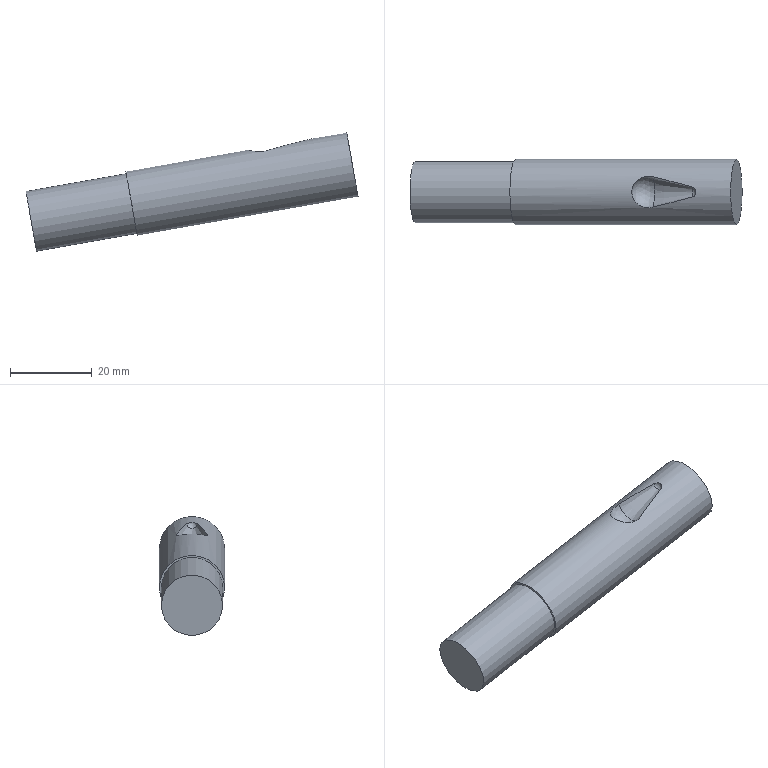Part | NX | features solid 2 | 1 solid | 8 faces | box 81.476 x 16 x 29.156 mm | volume 15288 mm3 | plane 3 | cylinder 2 | sphere 2 | cone 1 | commonest cylinder face diameters 15 x1 16 x1
STEP:
#1=CARTESIAN_POINT('',(-459.592,-11.393,50.494));
#2=VERTEX_POINT('',#1);
#3=CARTESIAN_POINT('',(-449.889,-8.922,53.051));
#4=VERTEX_POINT('',#3);
#5=CARTESIAN_POINT('',(-459.592,-11.393,50.494));
#6=CARTESIAN_POINT('',(-456.385,-10.61,51.483));
#7=CARTESIAN_POINT('',(-453.15,-9.775,52.335));
#8=CARTESIAN_POINT('',(-449.889,-8.922,53.051));
#9=B_SPLINE_CURVE_WITH_KNOTS('',3,(#5,#6,#7,#8),.UNSPECIFIED.,.F.,.F.,(4,4),(0.000000207,0.01034),.UNSPECIFIED.);
#10=EDGE_CURVE('',#2,#4,#9,.T.);
#11=ORIENTED_EDGE('',*,*,#10,.F.);
#12=CARTESIAN_POINT('',(-459.592,-3.877,50.494));
#13=VERTEX_POINT('',#12);
#14=CARTESIAN_POINT('',(-459.592,-3.877,50.494));
#15=CARTESIAN_POINT('',(-460.738,-3.598,50.141));
#16=CARTESIAN_POINT('',(-462.709,-3.96,50.065));
#17=CARTESIAN_POINT('',(-464.373,-5.808,50.453));
#18=CARTESIAN_POINT('',(-464.832,-7.629,50.597));
#19=CARTESIAN_POINT('',(-464.374,-9.46,50.454));
#20=CARTESIAN_POINT('',(-462.714,-11.307,50.066));
#21=CARTESIAN_POINT('',(-460.739,-11.672,50.141));
#22=CARTESIAN_POINT('',(-459.592,-11.393,50.494));
#23=B_SPLINE_CURVE_WITH_KNOTS('',3,(#14,#15,#16,#17,#18,#19,#20,#21,#22),.UNSPECIFIED.,.F.,.F.,(4,1,1,1,1,1,4),(0.000000204,0.003641,0.005462,0.007282,0.009103,0.01092,0.01456),.UNSPECIFIED.);
#24=EDGE_CURVE('',#13,#2,#23,.T.);
#25=ORIENTED_EDGE('',*,*,#24,.F.);
#26=CARTESIAN_POINT('',(-449.889,-6.348,53.051));
#27=VERTEX_POINT('',#26);
#28=CARTESIAN_POINT('',(-449.889,-6.348,53.051));
#29=CARTESIAN_POINT('',(-453.151,-5.495,52.335));
#30=CARTESIAN_POINT('',(-456.384,-4.66,51.483));
#31=CARTESIAN_POINT('',(-459.592,-3.877,50.494));
#32=B_SPLINE_CURVE_WITH_KNOTS('',3,(#28,#29,#30,#31),.UNSPECIFIED.,.F.,.F.,(4,4),(0.000000207,0.01034),.UNSPECIFIED.);
#33=EDGE_CURVE('',#27,#13,#32,.T.);
#34=ORIENTED_EDGE('',*,*,#33,.F.);
#35=CARTESIAN_POINT('',(-449.889,-8.922,53.051));
#36=CARTESIAN_POINT('',(-449.329,-8.775,53.174));
#37=CARTESIAN_POINT('',(-448.515,-7.637,53.481));
#38=CARTESIAN_POINT('',(-449.329,-6.494,53.174));
#39=CARTESIAN_POINT('',(-449.889,-6.348,53.051));
#40=B_SPLINE_CURVE_WITH_KNOTS('',3,(#35,#36,#37,#38,#39),.UNSPECIFIED.,.F.,.F.,(4,1,4),(0.000000204,0.00175,0.003499),.UNSPECIFIED.);
#41=EDGE_CURVE('',#4,#27,#40,.T.);
#42=ORIENTED_EDGE('',*,*,#41,.F.);
#43=EDGE_LOOP('',(#11,#25,#34,#42));
#44=FACE_BOUND('',#43,.T.);
#45=CARTESIAN_POINT('',(-438.998,-15.635,46.954));
#46=VERTEX_POINT('',#45);
#47=CARTESIAN_POINT('',(-438.998,-7.635,46.954));
#48=DIRECTION('',(-0.9848,0.,-0.1736));
#49=DIRECTION('',(0.,-1.,0.));
#50=AXIS2_PLACEMENT_3D('',#47,#48,#49);
#51=CIRCLE('',#50,8.);
#52=EDGE_CURVE('',#46,#46,#51,.T.);
#53=ORIENTED_EDGE('',*,*,#52,.T.);
#54=EDGE_LOOP('',(#53));
#55=FACE_BOUND('',#54,.T.);
#56=CARTESIAN_POINT('',(-493.163,-15.635,37.404));
#57=VERTEX_POINT('',#56);
#58=CARTESIAN_POINT('',(-493.163,-7.635,37.404));
#59=DIRECTION('',(-0.9848,0.,-0.1736));
#60=DIRECTION('',(0.,-1.,0.));
#61=AXIS2_PLACEMENT_3D('',#58,#59,#60);
#62=CIRCLE('',#61,8.);
#63=EDGE_CURVE('',#57,#57,#62,.T.);
#64=ORIENTED_EDGE('',*,*,#63,.F.);
#65=EDGE_LOOP('',(#64));
#66=FACE_BOUND('',#65,.T.);
#67=CARTESIAN_POINT('',(-438.998,-7.635,46.954));
#68=DIRECTION('',(-0.9848,0.,-0.1736));
#69=DIRECTION('',(0.,1.,0.));
#70=AXIS2_PLACEMENT_3D('',#67,#68,#69);
#71=CYLINDRICAL_SURFACE('',#70,8.);
#72=ADVANCED_FACE('',(#44,#55,#66),#71,.T.);
#73=ORIENTED_EDGE('',*,*,#52,.F.);
#74=EDGE_LOOP('',(#73));
#75=FACE_BOUND('',#74,.T.);
#76=CARTESIAN_POINT('',(-438.998,-7.635,46.954));
#77=DIRECTION('',(0.9848,0.,0.1736));
#78=DIRECTION('',(0.,-1.,0.));
#79=AXIS2_PLACEMENT_3D('',#76,#77,#78);
#80=PLANE('',#79);
#81=ADVANCED_FACE('',(#75),#80,.T.);
#82=CARTESIAN_POINT('',(-493.163,-15.135,37.404));
#83=VERTEX_POINT('',#82);
#84=CARTESIAN_POINT('',(-493.163,-7.635,37.404));
#85=DIRECTION('',(-0.9848,0.,-0.1736));
#86=DIRECTION('',(0.,-1.,0.));
#87=AXIS2_PLACEMENT_3D('',#84,#85,#86);
#88=CIRCLE('',#87,7.5);
#89=EDGE_CURVE('',#83,#83,#88,.T.);
#90=ORIENTED_EDGE('',*,*,#89,.F.);
#91=EDGE_LOOP('',(#90));
#92=FACE_BOUND('',#91,.T.);
#93=ORIENTED_EDGE('',*,*,#63,.T.);
#94=EDGE_LOOP('',(#93));
#95=FACE_BOUND('',#94,.T.);
#96=CARTESIAN_POINT('',(-493.163,-7.635,37.404));
#97=DIRECTION('',(0.9848,0.,0.1736));
#98=DIRECTION('',(0.,-1.,0.));
#99=AXIS2_PLACEMENT_3D('',#96,#97,#98);
#100=PLANE('',#99);
#101=ADVANCED_FACE('',(#92,#95),#100,.F.);
#102=CARTESIAN_POINT('',(-517.783,-15.135,33.062));
#103=VERTEX_POINT('',#102);
#104=CARTESIAN_POINT('',(-517.783,-7.635,33.062));
#105=DIRECTION('',(-0.9848,0.,-0.1736));
#106=DIRECTION('',(0.,-1.,0.));
#107=AXIS2_PLACEMENT_3D('',#104,#105,#106);
#108=CIRCLE('',#107,7.5);
#109=EDGE_CURVE('',#103,#103,#108,.T.);
#110=ORIENTED_EDGE('',*,*,#109,.F.);
#111=EDGE_LOOP('',(#110));
#112=FACE_BOUND('',#111,.T.);
#113=ORIENTED_EDGE('',*,*,#89,.T.);
#114=EDGE_LOOP('',(#113));
#115=FACE_BOUND('',#114,.T.);
#116=CARTESIAN_POINT('',(-517.783,-7.635,33.062));
#117=DIRECTION('',(0.9848,0.,0.1736));
#118=DIRECTION('',(0.,-1.,0.));
#119=AXIS2_PLACEMENT_3D('',#116,#117,#118);
#120=CYLINDRICAL_SURFACE('',#119,7.5);
#121=ADVANCED_FACE('',(#112,#115),#120,.T.);
#122=ORIENTED_EDGE('',*,*,#109,.T.);
#123=EDGE_LOOP('',(#122));
#124=FACE_BOUND('',#123,.T.);
#125=CARTESIAN_POINT('',(-517.783,-7.635,33.062));
#126=DIRECTION('',(0.9848,0.,0.1736));
#127=DIRECTION('',(0.,-1.,0.));
#128=AXIS2_PLACEMENT_3D('',#125,#126,#127);
#129=PLANE('',#128);
#130=ADVANCED_FACE('',(#124),#129,.F.);
#131=CARTESIAN_POINT('',(-459.755,-7.635,51.418));
#132=DIRECTION('',(0.9848,0.,0.1736));
#133=DIRECTION('',(0.,1.,0.));
#134=AXIS2_PLACEMENT_3D('',#131,#132,#133);
#135=CIRCLE('',#134,3.873);
#136=EDGE_CURVE('',#2,#13,#135,.T.);
#137=ORIENTED_EDGE('',*,*,#136,.T.);
#138=ORIENTED_EDGE('',*,*,#24,.T.);
#139=EDGE_LOOP('',(#137,#138));
#140=FACE_BOUND('',#139,.T.);
#141=CARTESIAN_POINT('',(-460.74,-7.635,51.244));
#142=DIRECTION('',(-0.9848,0.,-0.1736));
#143=DIRECTION('',(0.,1.,0.));
#144=AXIS2_PLACEMENT_3D('',#141,#142,#143);
#145=SPHERICAL_SURFACE('',#144,4.);
#146=ADVANCED_FACE('',(#140),#145,.F.);
#147=CARTESIAN_POINT('',(-449.907,-7.635,53.154));
#148=DIRECTION('',(0.9848,0.,0.1736));
#149=DIRECTION('',(0.,1.,0.));
#150=AXIS2_PLACEMENT_3D('',#147,#148,#149);
#151=CIRCLE('',#150,1.291);
#152=EDGE_CURVE('',#4,#27,#151,.T.);
#153=ORIENTED_EDGE('',*,*,#152,.T.);
#154=ORIENTED_EDGE('',*,*,#33,.T.);
#155=ORIENTED_EDGE('',*,*,#136,.F.);
#156=ORIENTED_EDGE('',*,*,#10,.T.);
#157=EDGE_LOOP('',(#153,#154,#155,#156));
#158=FACE_BOUND('',#157,.T.);
#159=CARTESIAN_POINT('',(-459.755,-7.635,51.418));
#160=DIRECTION('',(-0.9848,0.,-0.1736));
#161=DIRECTION('',(0.,1.,0.));
#162=AXIS2_PLACEMENT_3D('',#159,#160,#161);
#163=CONICAL_SURFACE('',#162,3.873,0.2527);
#164=ADVANCED_FACE('',(#158),#163,.F.);
#165=ORIENTED_EDGE('',*,*,#152,.F.);
#166=ORIENTED_EDGE('',*,*,#41,.T.);
#167=EDGE_LOOP('',(#165,#166));
#168=FACE_BOUND('',#167,.T.);
#169=CARTESIAN_POINT('',(-450.235,-7.635,53.096));
#170=DIRECTION('',(-0.9848,0.,-0.1736));
#171=DIRECTION('',(0.,-1.,0.));
#172=AXIS2_PLACEMENT_3D('',#169,#170,#171);
#173=SPHERICAL_SURFACE('',#172,1.333);
#174=ADVANCED_FACE('',(#168),#173,.F.);
#175=CLOSED_SHELL('',(#72,#81,#101,#121,#130,#146,#164,#174));
#176=MANIFOLD_SOLID_BREP('',#175);
#177=(LENGTH_UNIT()NAMED_UNIT(*)SI_UNIT(.MILLI.,.METRE.));
#178=UNCERTAINTY_MEASURE_WITH_UNIT(LENGTH_MEASURE(0.0508),#177,'','');
#179=(NAMED_UNIT(*)PLANE_ANGLE_UNIT()SI_UNIT($,.RADIAN.));
#180=(NAMED_UNIT(*)SI_UNIT($,.STERADIAN.)SOLID_ANGLE_UNIT());
#181=(GEOMETRIC_REPRESENTATION_CONTEXT(3)GLOBAL_UNCERTAINTY_ASSIGNED_CONTEXT((#178))GLOBAL_UNIT_ASSIGNED_CONTEXT((#177,#179,#180))REPRESENTATION_CONTEXT('',''));
#182=ADVANCED_BREP_SHAPE_REPRESENTATION('',(#176),#181);